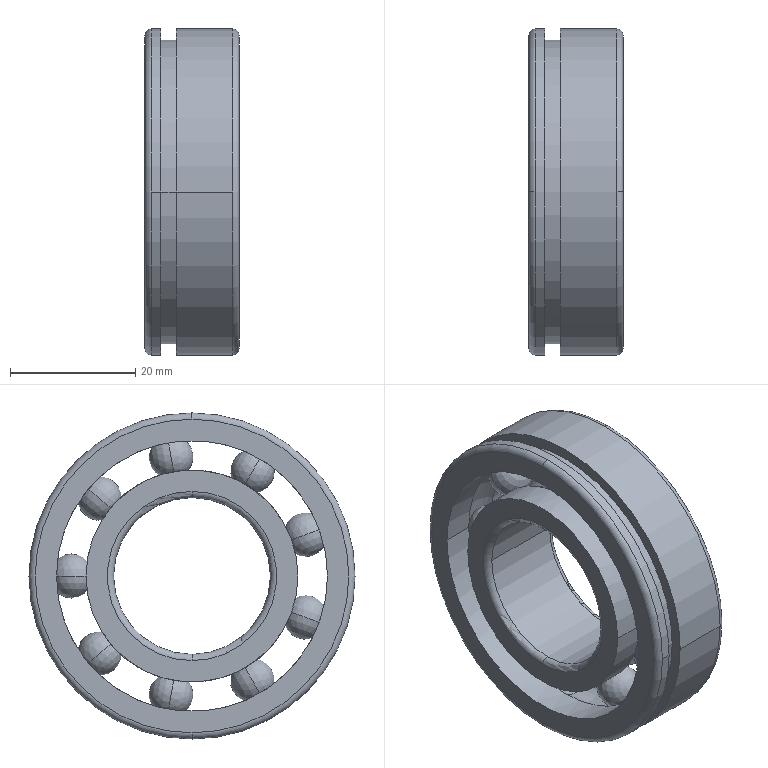Part | SolidWorks | features BaseBody 11 | 11 solids | 54 faces | box 15 x 52 x 52 mm | volume 15772 mm3 | sphere 18 | cylinder 16 | torus 14 | plane 6 | commonest cylinder face diameters 33.802 x4 43.198 x4 52 x4 25 x2 48.4 x2
STEP:
#1=CARTESIAN_POINT('',(7.5,15.74,0.));
#2=VERTEX_POINT('',#1);
#3=CARTESIAN_POINT('',(7.5,22.76,0.));
#4=VERTEX_POINT('',#3);
#5=CARTESIAN_POINT('',(7.5,19.25,0.));
#6=DIRECTION('',(0.,0.,1.));
#7=DIRECTION('',(1.,0.,0.));
#8=AXIS2_PLACEMENT_3D('',#5,#6,#7);
#9=CIRCLE('',#8,3.51);
#10=EDGE_CURVE('',#2,#4,#9,.T.);
#11=ORIENTED_EDGE('',*,*,#10,.F.);
#12=CARTESIAN_POINT('',(7.5,19.25,0.));
#13=DIRECTION('',(0.,0.,-1.));
#14=DIRECTION('',(-1.,0.,0.));
#15=AXIS2_PLACEMENT_3D('',#12,#13,#14);
#16=CIRCLE('',#15,3.51);
#17=EDGE_CURVE('',#2,#4,#16,.T.);
#18=ORIENTED_EDGE('',*,*,#17,.T.);
#19=EDGE_LOOP('',(#11,#18));
#20=FACE_OUTER_BOUND('',#19,.T.);
#21=CARTESIAN_POINT('',(7.5,19.25,0.));
#22=DIRECTION('',(0.,0.,-1.));
#23=DIRECTION('',(1.,0.,0.));
#24=AXIS2_PLACEMENT_3D('',#21,#22,#23);
#25=SPHERICAL_SURFACE('',#24,3.51);
#26=ADVANCED_FACE('',(#20),#25,.T.);
#27=ORIENTED_EDGE('',*,*,#17,.F.);
#28=ORIENTED_EDGE('',*,*,#10,.T.);
#29=EDGE_LOOP('',(#27,#28));
#30=FACE_OUTER_BOUND('',#29,.T.);
#31=CARTESIAN_POINT('',(7.5,19.25,0.));
#32=DIRECTION('',(0.,0.,-1.));
#33=DIRECTION('',(1.,0.,0.));
#34=AXIS2_PLACEMENT_3D('',#31,#32,#33);
#35=SPHERICAL_SURFACE('',#34,3.51);
#36=ADVANCED_FACE('',(#30),#35,.T.);
#37=CLOSED_SHELL('',(#26,#36));
#38=MANIFOLD_SOLID_BREP('',#37);
#39=CARTESIAN_POINT('',(5.,-24.2,0.));
#40=VERTEX_POINT('',#39);
#41=CARTESIAN_POINT('',(5.,24.2,0.));
#42=VERTEX_POINT('',#41);
#43=CARTESIAN_POINT('',(5.,0.,0.));
#44=DIRECTION('',(1.,0.,0.));
#45=DIRECTION('',(0.,1.,0.));
#46=AXIS2_PLACEMENT_3D('',#43,#44,#45);
#47=CIRCLE('',#46,24.2);
#48=EDGE_CURVE('',#40,#42,#47,.T.);
#49=ORIENTED_EDGE('',*,*,#48,.F.);
#50=CARTESIAN_POINT('',(2.5,-24.2,0.));
#51=VERTEX_POINT('',#50);
#52=CARTESIAN_POINT('',(3.75,-24.2,0.));
#53=DIRECTION('',(-1.,0.,0.));
#54=VECTOR('',#53,1000.);
#55=LINE('',#52,#54);
#56=EDGE_CURVE('',#40,#51,#55,.T.);
#57=ORIENTED_EDGE('',*,*,#56,.T.);
#58=CARTESIAN_POINT('',(2.5,24.2,0.));
#59=VERTEX_POINT('',#58);
#60=CARTESIAN_POINT('',(2.5,0.,0.));
#61=DIRECTION('',(1.,0.,0.));
#62=DIRECTION('',(0.,1.,0.));
#63=AXIS2_PLACEMENT_3D('',#60,#61,#62);
#64=CIRCLE('',#63,24.2);
#65=EDGE_CURVE('',#51,#59,#64,.T.);
#66=ORIENTED_EDGE('',*,*,#65,.T.);
#67=CARTESIAN_POINT('',(3.75,24.2,0.));
#68=DIRECTION('',(-1.,0.,0.));
#69=VECTOR('',#68,1000.);
#70=LINE('',#67,#69);
#71=EDGE_CURVE('',#42,#59,#70,.T.);
#72=ORIENTED_EDGE('',*,*,#71,.F.);
#73=EDGE_LOOP('',(#49,#57,#66,#72));
#74=FACE_OUTER_BOUND('',#73,.T.);
#75=CARTESIAN_POINT('',(3.75,0.,0.));
#76=DIRECTION('',(-1.,0.,0.));
#77=DIRECTION('',(0.,1.,0.));
#78=AXIS2_PLACEMENT_3D('',#75,#76,#77);
#79=CYLINDRICAL_SURFACE('',#78,24.2);
#80=ADVANCED_FACE('',(#74),#79,.T.);
#81=CARTESIAN_POINT('',(14.,-26.,0.));
#82=VERTEX_POINT('',#81);
#83=CARTESIAN_POINT('',(14.,0.,-26.));
#84=VERTEX_POINT('',#83);
#85=CARTESIAN_POINT('',(14.,0.,0.));
#86=DIRECTION('',(1.,0.,0.));
#87=DIRECTION('',(0.,-1.,0.));
#88=AXIS2_PLACEMENT_3D('',#85,#86,#87);
#89=CIRCLE('',#88,26.);
#90=EDGE_CURVE('',#82,#84,#89,.T.);
#91=ORIENTED_EDGE('',*,*,#90,.F.);
#92=CARTESIAN_POINT('',(5.,-26.,0.));
#93=VERTEX_POINT('',#92);
#94=CARTESIAN_POINT('',(10.,-26.,0.));
#95=DIRECTION('',(-1.,0.,0.));
#96=VECTOR('',#95,1000.);
#97=LINE('',#94,#96);
#98=EDGE_CURVE('',#82,#93,#97,.T.);
#99=ORIENTED_EDGE('',*,*,#98,.T.);
#100=CARTESIAN_POINT('',(5.,26.,0.));
#101=VERTEX_POINT('',#100);
#102=CARTESIAN_POINT('',(5.,0.,0.));
#103=DIRECTION('',(1.,0.,0.));
#104=DIRECTION('',(0.,1.,0.));
#105=AXIS2_PLACEMENT_3D('',#102,#103,#104);
#106=CIRCLE('',#105,26.);
#107=EDGE_CURVE('',#93,#101,#106,.T.);
#108=ORIENTED_EDGE('',*,*,#107,.T.);
#109=CARTESIAN_POINT('',(14.,26.,0.));
#110=VERTEX_POINT('',#109);
#111=CARTESIAN_POINT('',(10.,26.,0.));
#112=DIRECTION('',(-1.,0.,0.));
#113=VECTOR('',#112,1000.);
#114=LINE('',#111,#113);
#115=EDGE_CURVE('',#110,#101,#114,.T.);
#116=ORIENTED_EDGE('',*,*,#115,.F.);
#117=CARTESIAN_POINT('',(14.,0.,0.));
#118=DIRECTION('',(1.,0.,0.));
#119=DIRECTION('',(0.,-1.,0.));
#120=AXIS2_PLACEMENT_3D('',#117,#118,#119);
#121=CIRCLE('',#120,26.);
#122=EDGE_CURVE('',#84,#110,#121,.T.);
#123=ORIENTED_EDGE('',*,*,#122,.F.);
#124=EDGE_LOOP('',(#91,#99,#108,#116,#123));
#125=FACE_OUTER_BOUND('',#124,.T.);
#126=CARTESIAN_POINT('',(10.,0.,0.));
#127=DIRECTION('',(-1.,0.,0.));
#128=DIRECTION('',(0.,1.,0.));
#129=AXIS2_PLACEMENT_3D('',#126,#127,#128);
#130=CYLINDRICAL_SURFACE('',#129,26.);
#131=ADVANCED_FACE('',(#125),#130,.T.);
#132=CARTESIAN_POINT('',(2.5,-26.,0.));
#133=VERTEX_POINT('',#132);
#134=CARTESIAN_POINT('',(2.5,26.,0.));
#135=VERTEX_POINT('',#134);
#136=CARTESIAN_POINT('',(2.5,0.,0.));
#137=DIRECTION('',(1.,0.,0.));
#138=DIRECTION('',(0.,1.,0.));
#139=AXIS2_PLACEMENT_3D('',#136,#137,#138);
#140=CIRCLE('',#139,26.);
#141=EDGE_CURVE('',#133,#135,#140,.T.);
#142=ORIENTED_EDGE('',*,*,#141,.F.);
#143=CARTESIAN_POINT('',(1.,-26.,0.));
#144=VERTEX_POINT('',#143);
#145=CARTESIAN_POINT('',(1.25,-26.,0.));
#146=DIRECTION('',(-1.,0.,0.));
#147=VECTOR('',#146,1000.);
#148=LINE('',#145,#147);
#149=EDGE_CURVE('',#133,#144,#148,.T.);
#150=ORIENTED_EDGE('',*,*,#149,.T.);
#151=CARTESIAN_POINT('',(1.,0.,-26.));
#152=VERTEX_POINT('',#151);
#153=CARTESIAN_POINT('',(1.,0.,0.));
#154=DIRECTION('',(-1.,0.,0.));
#155=DIRECTION('',(0.,-1.,0.));
#156=AXIS2_PLACEMENT_3D('',#153,#154,#155);
#157=CIRCLE('',#156,26.);
#158=EDGE_CURVE('',#152,#144,#157,.T.);
#159=ORIENTED_EDGE('',*,*,#158,.F.);
#160=CARTESIAN_POINT('',(1.,26.,0.));
#161=VERTEX_POINT('',#160);
#162=CARTESIAN_POINT('',(1.,0.,0.));
#163=DIRECTION('',(-1.,0.,0.));
#164=DIRECTION('',(0.,-1.,0.));
#165=AXIS2_PLACEMENT_3D('',#162,#163,#164);
#166=CIRCLE('',#165,26.);
#167=EDGE_CURVE('',#161,#152,#166,.T.);
#168=ORIENTED_EDGE('',*,*,#167,.F.);
#169=CARTESIAN_POINT('',(1.25,26.,0.));
#170=DIRECTION('',(-1.,0.,0.));
#171=VECTOR('',#170,1000.);
#172=LINE('',#169,#171);
#173=EDGE_CURVE('',#135,#161,#172,.T.);
#174=ORIENTED_EDGE('',*,*,#173,.F.);
#175=EDGE_LOOP('',(#142,#150,#159,#168,#174));
#176=FACE_OUTER_BOUND('',#175,.T.);
#177=CARTESIAN_POINT('',(1.25,0.,0.));
#178=DIRECTION('',(-1.,0.,0.));
#179=DIRECTION('',(0.,1.,0.));
#180=AXIS2_PLACEMENT_3D('',#177,#178,#179);
#181=CYLINDRICAL_SURFACE('',#180,26.);
#182=ADVANCED_FACE('',(#176),#181,.T.);
#183=ORIENTED_EDGE('',*,*,#122,.T.);
#184=CARTESIAN_POINT('',(14.,0.,26.));
#185=VERTEX_POINT('',#184);
#186=CARTESIAN_POINT('',(14.,0.,0.));
#187=DIRECTION('',(1.,0.,0.));
#188=DIRECTION('',(0.,-1.,0.));
#189=AXIS2_PLACEMENT_3D('',#186,#187,#188);
#190=CIRCLE('',#189,26.);
#191=EDGE_CURVE('',#110,#185,#190,.T.);
#192=ORIENTED_EDGE('',*,*,#191,.T.);
#193=CARTESIAN_POINT('',(15.,0.,25.));
#194=VERTEX_POINT('',#193);
#195=CARTESIAN_POINT('',(14.,0.,25.));
#196=DIRECTION('',(0.,1.,0.));
#197=DIRECTION('',(0.,0.,1.));
#198=AXIS2_PLACEMENT_3D('',#195,#196,#197);
#199=CIRCLE('',#198,1.);
#200=EDGE_CURVE('',#185,#194,#199,.T.);
#201=ORIENTED_EDGE('',*,*,#200,.T.);
#202=CARTESIAN_POINT('',(15.,0.,-25.));
#203=VERTEX_POINT('',#202);
#204=CARTESIAN_POINT('',(15.,0.,0.));
#205=DIRECTION('',(-1.,0.,0.));
#206=DIRECTION('',(0.,-1.,0.));
#207=AXIS2_PLACEMENT_3D('',#204,#205,#206);
#208=CIRCLE('',#207,25.);
#209=EDGE_CURVE('',#194,#203,#208,.T.);
#210=ORIENTED_EDGE('',*,*,#209,.T.);
#211=CARTESIAN_POINT('',(14.,0.,-25.));
#212=DIRECTION('',(0.,-1.,0.));
#213=DIRECTION('',(0.,0.,-1.));
#214=AXIS2_PLACEMENT_3D('',#211,#212,#213);
#215=CIRCLE('',#214,1.);
#216=EDGE_CURVE('',#84,#203,#215,.T.);
#217=ORIENTED_EDGE('',*,*,#216,.F.);
#218=EDGE_LOOP('',(#183,#192,#201,#210,#217));
#219=FACE_OUTER_BOUND('',#218,.T.);
#220=CARTESIAN_POINT('',(14.,0.,0.));
#221=DIRECTION('',(1.,0.,0.));
#222=DIRECTION('',(0.,0.,-1.));
#223=AXIS2_PLACEMENT_3D('',#220,#221,#222);
#224=TOROIDAL_SURFACE('',#223,25.,1.);
#225=ADVANCED_FACE('',(#219),#224,.T.);
#226=CARTESIAN_POINT('',(0.,0.,-25.));
#227=VERTEX_POINT('',#226);
#228=CARTESIAN_POINT('',(0.,0.,25.));
#229=VERTEX_POINT('',#228);
#230=CARTESIAN_POINT('',(0.,0.,0.));
#231=DIRECTION('',(1.,0.,0.));
#232=DIRECTION('',(0.,-1.,0.));
#233=AXIS2_PLACEMENT_3D('',#230,#231,#232);
#234=CIRCLE('',#233,25.);
#235=EDGE_CURVE('',#227,#229,#234,.T.);
#236=ORIENTED_EDGE('',*,*,#235,.T.);
#237=CARTESIAN_POINT('',(1.,0.,26.));
#238=VERTEX_POINT('',#237);
#239=CARTESIAN_POINT('',(1.,0.,25.));
#240=DIRECTION('',(0.,1.,0.));
#241=DIRECTION('',(0.,0.,1.));
#242=AXIS2_PLACEMENT_3D('',#239,#240,#241);
#243=CIRCLE('',#242,1.);
#244=EDGE_CURVE('',#229,#238,#243,.T.);
#245=ORIENTED_EDGE('',*,*,#244,.T.);
#246=CARTESIAN_POINT('',(1.,0.,0.));
#247=DIRECTION('',(-1.,0.,0.));
#248=DIRECTION('',(0.,-1.,0.));
#249=AXIS2_PLACEMENT_3D('',#246,#247,#248);
#250=CIRCLE('',#249,26.);
#251=EDGE_CURVE('',#238,#161,#250,.T.);
#252=ORIENTED_EDGE('',*,*,#251,.T.);
#253=ORIENTED_EDGE('',*,*,#167,.T.);
#254=CARTESIAN_POINT('',(1.,0.,-25.));
#255=DIRECTION('',(0.,-1.,0.));
#256=DIRECTION('',(0.,0.,-1.));
#257=AXIS2_PLACEMENT_3D('',#254,#255,#256);
#258=CIRCLE('',#257,1.);
#259=EDGE_CURVE('',#227,#152,#258,.T.);
#260=ORIENTED_EDGE('',*,*,#259,.F.);
#261=EDGE_LOOP('',(#236,#245,#252,#253,#260));
#262=FACE_OUTER_BOUND('',#261,.T.);
#263=CARTESIAN_POINT('',(1.,0.,0.));
#264=DIRECTION('',(1.,0.,0.));
#265=DIRECTION('',(0.,0.,-1.));
#266=AXIS2_PLACEMENT_3D('',#263,#264,#265);
#267=TOROIDAL_SURFACE('',#266,25.,1.);
#268=ADVANCED_FACE('',(#262),#267,.T.);
#269=CARTESIAN_POINT('',(4.892,0.,21.599));
#270=VERTEX_POINT('',#269);
#271=CARTESIAN_POINT('',(4.892,-21.599,0.));
#272=VERTEX_POINT('',#271);
#273=CARTESIAN_POINT('',(4.892,0.,0.));
#274=DIRECTION('',(1.,0.,0.));
#275=DIRECTION('',(0.,1.,0.));
#276=AXIS2_PLACEMENT_3D('',#273,#274,#275);
#277=CIRCLE('',#276,21.599);
#278=EDGE_CURVE('',#270,#272,#277,.T.);
#279=ORIENTED_EDGE('',*,*,#278,.F.);
#280=CARTESIAN_POINT('',(10.108,0.,21.599));
#281=VERTEX_POINT('',#280);
#282=CARTESIAN_POINT('',(7.5,0.,19.25));
#283=DIRECTION('',(0.,1.,0.));
#284=DIRECTION('',(0.,0.,1.));
#285=AXIS2_PLACEMENT_3D('',#282,#283,#284);
#286=CIRCLE('',#285,3.51);
#287=EDGE_CURVE('',#270,#281,#286,.T.);
#288=ORIENTED_EDGE('',*,*,#287,.T.);
#289=CARTESIAN_POINT('',(10.108,-21.599,0.));
#290=VERTEX_POINT('',#289);
#291=CARTESIAN_POINT('',(10.108,0.,0.));
#292=DIRECTION('',(1.,0.,0.));
#293=DIRECTION('',(0.,1.,0.));
#294=AXIS2_PLACEMENT_3D('',#291,#292,#293);
#295=CIRCLE('',#294,21.599);
#296=EDGE_CURVE('',#281,#290,#295,.T.);
#297=ORIENTED_EDGE('',*,*,#296,.T.);
#298=CARTESIAN_POINT('',(10.108,0.,-21.599));
#299=VERTEX_POINT('',#298);
#300=CARTESIAN_POINT('',(10.108,0.,0.));
#301=DIRECTION('',(1.,0.,0.));
#302=DIRECTION('',(0.,1.,0.));
#303=AXIS2_PLACEMENT_3D('',#300,#301,#302);
#304=CIRCLE('',#303,21.599);
#305=EDGE_CURVE('',#290,#299,#304,.T.);
#306=ORIENTED_EDGE('',*,*,#305,.T.);
#307=CARTESIAN_POINT('',(4.892,0.,-21.599));
#308=VERTEX_POINT('',#307);
#309=CARTESIAN_POINT('',(7.5,0.,-19.25));
#310=DIRECTION('',(0.,-1.,0.));
#311=DIRECTION('',(0.,0.,-1.));
#312=AXIS2_PLACEMENT_3D('',#309,#310,#311);
#313=CIRCLE('',#312,3.51);
#314=EDGE_CURVE('',#308,#299,#313,.T.);
#315=ORIENTED_EDGE('',*,*,#314,.F.);
#316=CARTESIAN_POINT('',(4.892,0.,0.));
#317=DIRECTION('',(1.,0.,0.));
#318=DIRECTION('',(0.,1.,0.));
#319=AXIS2_PLACEMENT_3D('',#316,#317,#318);
#320=CIRCLE('',#319,21.599);
#321=EDGE_CURVE('',#272,#308,#320,.T.);
#322=ORIENTED_EDGE('',*,*,#321,.F.);
#323=EDGE_LOOP('',(#279,#288,#297,#306,#315,#322));
#324=FACE_OUTER_BOUND('',#323,.T.);
#325=CARTESIAN_POINT('',(7.5,0.,0.));
#326=DIRECTION('',(1.,0.,0.));
#327=DIRECTION('',(0.,0.,-1.));
#328=AXIS2_PLACEMENT_3D('',#325,#326,#327);
#329=TOROIDAL_SURFACE('',#328,19.25,3.51);
#330=ADVANCED_FACE('',(#324),#329,.F.);
#331=CARTESIAN_POINT('',(15.,21.599,0.));
#332=VERTEX_POINT('',#331);
#333=CARTESIAN_POINT('',(15.,-21.599,0.));
#334=VERTEX_POINT('',#333);
#335=CARTESIAN_POINT('',(15.,0.,0.));
#336=DIRECTION('',(1.,0.,0.));
#337=DIRECTION('',(0.,1.,0.));
#338=AXIS2_PLACEMENT_3D('',#335,#336,#337);
#339=CIRCLE('',#338,21.599);
#340=EDGE_CURVE('',#332,#334,#339,.T.);
#341=ORIENTED_EDGE('',*,*,#340,.T.);
#342=CARTESIAN_POINT('',(12.554,-21.599,0.));
#343=DIRECTION('',(-1.,0.,0.));
#344=VECTOR('',#343,1000.);
#345=LINE('',#342,#344);
#346=EDGE_CURVE('',#334,#290,#345,.T.);
#347=ORIENTED_EDGE('',*,*,#346,.T.);
#348=ORIENTED_EDGE('',*,*,#296,.F.);
#349=CARTESIAN_POINT('',(10.108,21.599,0.));
#350=VERTEX_POINT('',#349);
#351=CARTESIAN_POINT('',(10.108,0.,0.));
#352=DIRECTION('',(1.,0.,0.));
#353=DIRECTION('',(0.,1.,0.));
#354=AXIS2_PLACEMENT_3D('',#351,#352,#353);
#355=CIRCLE('',#354,21.599);
#356=EDGE_CURVE('',#350,#281,#355,.T.);
#357=ORIENTED_EDGE('',*,*,#356,.F.);
#358=CARTESIAN_POINT('',(12.554,21.599,0.));
#359=DIRECTION('',(-1.,0.,0.));
#360=VECTOR('',#359,1000.);
#361=LINE('',#358,#360);
#362=EDGE_CURVE('',#332,#350,#361,.T.);
#363=ORIENTED_EDGE('',*,*,#362,.F.);
#364=EDGE_LOOP('',(#341,#347,#348,#357,#363));
#365=FACE_OUTER_BOUND('',#364,.T.);
#366=CARTESIAN_POINT('',(12.554,0.,0.));
#367=DIRECTION('',(-1.,0.,0.));
#368=DIRECTION('',(0.,1.,0.));
#369=AXIS2_PLACEMENT_3D('',#366,#367,#368);
#370=CYLINDRICAL_SURFACE('',#369,21.599);
#371=ADVANCED_FACE('',(#365),#370,.F.);
#372=CARTESIAN_POINT('',(4.892,21.599,0.));
#373=VERTEX_POINT('',#372);
#374=CARTESIAN_POINT('',(4.892,0.,0.));
#375=DIRECTION('',(1.,0.,0.));
#376=DIRECTION('',(0.,1.,0.));
#377=AXIS2_PLACEMENT_3D('',#374,#375,#376);
#378=CIRCLE('',#377,21.599);
#379=EDGE_CURVE('',#373,#270,#378,.T.);
#380=ORIENTED_EDGE('',*,*,#379,.T.);
#381=ORIENTED_EDGE('',*,*,#278,.T.);
#382=CARTESIAN_POINT('',(0.,-21.599,0.));
#383=VERTEX_POINT('',#382);
#384=CARTESIAN_POINT('',(2.446,-21.599,0.));
#385=DIRECTION('',(-1.,0.,0.));
#386=VECTOR('',#385,1000.);
#387=LINE('',#384,#386);
#388=EDGE_CURVE('',#272,#383,#387,.T.);
#389=ORIENTED_EDGE('',*,*,#388,.T.);
#390=CARTESIAN_POINT('',(0.,21.599,0.));
#391=VERTEX_POINT('',#390);
#392=CARTESIAN_POINT('',(0.,0.,0.));
#393=DIRECTION('',(1.,0.,0.));
#394=DIRECTION('',(0.,1.,0.));
#395=AXIS2_PLACEMENT_3D('',#392,#393,#394);
#396=CIRCLE('',#395,21.599);
#397=EDGE_CURVE('',#391,#383,#396,.T.);
#398=ORIENTED_EDGE('',*,*,#397,.F.);
#399=CARTESIAN_POINT('',(2.446,21.599,0.));
#400=DIRECTION('',(-1.,0.,0.));
#401=VECTOR('',#400,1000.);
#402=LINE('',#399,#401);
#403=EDGE_CURVE('',#373,#391,#402,.T.);
#404=ORIENTED_EDGE('',*,*,#403,.F.);
#405=EDGE_LOOP('',(#380,#381,#389,#398,#404));
#406=FACE_OUTER_BOUND('',#405,.T.);
#407=CARTESIAN_POINT('',(2.446,0.,0.));
#408=DIRECTION('',(-1.,0.,0.));
#409=DIRECTION('',(0.,1.,0.));
#410=AXIS2_PLACEMENT_3D('',#407,#408,#409);
#411=CYLINDRICAL_SURFACE('',#410,21.599);
#412=ADVANCED_FACE('',(#406),#411,.F.);
#413=CARTESIAN_POINT('',(5.,0.,0.));
#414=DIRECTION('',(1.,0.,0.));
#415=DIRECTION('',(0.,1.,0.));
#416=AXIS2_PLACEMENT_3D('',#413,#414,#415);
#417=CIRCLE('',#416,24.2);
#418=EDGE_CURVE('',#42,#40,#417,.T.);
#419=ORIENTED_EDGE('',*,*,#418,.T.);
#420=ORIENTED_EDGE('',*,*,#48,.T.);
#421=EDGE_LOOP('',(#419,#420));
#422=FACE_BOUND('',#421,.T.);
#423=CARTESIAN_POINT('',(5.,0.,0.));
#424=DIRECTION('',(1.,0.,0.));
#425=DIRECTION('',(0.,1.,0.));
#426=AXIS2_PLACEMENT_3D('',#423,#424,#425);
#427=CIRCLE('',#426,26.);
#428=EDGE_CURVE('',#101,#93,#427,.T.);
#429=ORIENTED_EDGE('',*,*,#428,.F.);
#430=ORIENTED_EDGE('',*,*,#107,.F.);
#431=EDGE_LOOP('',(#429,#430));
#432=FACE_OUTER_BOUND('',#431,.T.);
#433=CARTESIAN_POINT('',(5.,25.1,0.));
#434=DIRECTION('',(-1.,0.,0.));
#435=DIRECTION('',(0.,0.,1.));
#436=AXIS2_PLACEMENT_3D('',#433,#434,#435);
#437=PLANE('',#436);
#438=ADVANCED_FACE('',(#422,#432),#437,.T.);
#439=CARTESIAN_POINT('',(2.5,0.,0.));
#440=DIRECTION('',(1.,0.,0.));
#441=DIRECTION('',(0.,1.,0.));
#442=AXIS2_PLACEMENT_3D('',#439,#440,#441);
#443=CIRCLE('',#442,24.2);
#444=EDGE_CURVE('',#59,#51,#443,.T.);
#445=ORIENTED_EDGE('',*,*,#444,.F.);
#446=ORIENTED_EDGE('',*,*,#65,.F.);
#447=EDGE_LOOP('',(#445,#446));
#448=FACE_BOUND('',#447,.T.);
#449=CARTESIAN_POINT('',(2.5,0.,0.));
#450=DIRECTION('',(1.,0.,0.));
#451=DIRECTION('',(0.,1.,0.));
#452=AXIS2_PLACEMENT_3D('',#449,#450,#451);
#453=CIRCLE('',#452,26.);
#454=EDGE_CURVE('',#135,#133,#453,.T.);
#455=ORIENTED_EDGE('',*,*,#454,.T.);
#456=ORIENTED_EDGE('',*,*,#141,.T.);
#457=EDGE_LOOP('',(#455,#456));
#458=FACE_OUTER_BOUND('',#457,.T.);
#459=CARTESIAN_POINT('',(2.5,25.1,0.));
#460=DIRECTION('',(1.,0.,0.));
#461=DIRECTION('',(0.,1.,0.));
#462=AXIS2_PLACEMENT_3D('',#459,#460,#461);
#463=PLANE('',#462);
#464=ADVANCED_FACE('',(#448,#458),#463,.T.);
#465=ORIENTED_EDGE('',*,*,#340,.F.);
#466=CARTESIAN_POINT('',(15.,0.,0.));
#467=DIRECTION('',(1.,0.,0.));
#468=DIRECTION('',(0.,1.,0.));
#469=AXIS2_PLACEMENT_3D('',#466,#467,#468);
#470=CIRCLE('',#469,21.599);
#471=EDGE_CURVE('',#334,#332,#470,.T.);
#472=ORIENTED_EDGE('',*,*,#471,.F.);
#473=EDGE_LOOP('',(#465,#472));
#474=FACE_BOUND('',#473,.T.);
#475=CARTESIAN_POINT('',(15.,0.,0.));
#476=DIRECTION('',(-1.,0.,0.));
#477=DIRECTION('',(0.,-1.,0.));
#478=AXIS2_PLACEMENT_3D('',#475,#476,#477);
#479=CIRCLE('',#478,25.);
#480=EDGE_CURVE('',#203,#194,#479,.T.);
#481=ORIENTED_EDGE('',*,*,#480,.F.);
#482=ORIENTED_EDGE('',*,*,#209,.F.);
#483=EDGE_LOOP('',(#481,#482));
#484=FACE_OUTER_BOUND('',#483,.T.);
#485=CARTESIAN_POINT('',(15.,23.8,0.));
#486=DIRECTION('',(1.,0.,0.));
#487=DIRECTION('',(0.,1.,0.));
#488=AXIS2_PLACEMENT_3D('',#485,#486,#487);
#489=PLANE('',#488);
#490=ADVANCED_FACE('',(#474,#484),#489,.T.);
#491=ORIENTED_EDGE('',*,*,#397,.T.);
#492=CARTESIAN_POINT('',(0.,0.,0.));
#493=DIRECTION('',(1.,0.,0.));
#494=DIRECTION('',(0.,1.,0.));
#495=AXIS2_PLACEMENT_3D('',#492,#493,#494);
#496=CIRCLE('',#495,21.599);
#497=EDGE_CURVE('',#383,#391,#496,.T.);
#498=ORIENTED_EDGE('',*,*,#497,.T.);
#499=EDGE_LOOP('',(#491,#498));
#500=FACE_BOUND('',#499,.T.);
#501=ORIENTED_EDGE('',*,*,#235,.F.);
#502=CARTESIAN_POINT('',(0.,0.,0.));
#503=DIRECTION('',(1.,0.,0.));
#504=DIRECTION('',(0.,-1.,0.));
#505=AXIS2_PLACEMENT_3D('',#502,#503,#504);
#506=CIRCLE('',#505,25.);
#507=EDGE_CURVE('',#229,#227,#506,.T.);
#508=ORIENTED_EDGE('',*,*,#507,.F.);
#509=EDGE_LOOP('',(#501,#508));
#510=FACE_OUTER_BOUND('',#509,.T.);
#511=CARTESIAN_POINT('',(0.,23.8,0.));
#512=DIRECTION('',(-1.,0.,0.));
#513=DIRECTION('',(0.,0.,1.));
#514=AXIS2_PLACEMENT_3D('',#511,#512,#513);
#515=PLANE('',#514);
#516=ADVANCED_FACE('',(#500,#510),#515,.T.);
#517=ORIENTED_EDGE('',*,*,#388,.F.);
#518=ORIENTED_EDGE('',*,*,#321,.T.);
#519=CARTESIAN_POINT('',(4.892,0.,0.));
#520=DIRECTION('',(1.,0.,0.));
#521=DIRECTION('',(0.,1.,0.));
#522=AXIS2_PLACEMENT_3D('',#519,#520,#521);
#523=CIRCLE('',#522,21.599);
#524=EDGE_CURVE('',#308,#373,#523,.T.);
#525=ORIENTED_EDGE('',*,*,#524,.T.);
#526=ORIENTED_EDGE('',*,*,#403,.T.);
#527=ORIENTED_EDGE('',*,*,#497,.F.);
#528=EDGE_LOOP('',(#517,#518,#525,#526,#527));
#529=FACE_OUTER_BOUND('',#528,.T.);
#530=CARTESIAN_POINT('',(2.446,0.,0.));
#531=DIRECTION('',(-1.,0.,0.));
#532=DIRECTION('',(0.,1.,0.));
#533=AXIS2_PLACEMENT_3D('',#530,#531,#532);
#534=CYLINDRICAL_SURFACE('',#533,21.599);
#535=ADVANCED_FACE('',(#529),#534,.F.);
#536=ORIENTED_EDGE('',*,*,#346,.F.);
#537=ORIENTED_EDGE('',*,*,#471,.T.);
#538=ORIENTED_EDGE('',*,*,#362,.T.);
#539=CARTESIAN_POINT('',(10.108,0.,0.));
#540=DIRECTION('',(1.,0.,0.));
#541=DIRECTION('',(0.,1.,0.));
#542=AXIS2_PLACEMENT_3D('',#539,#540,#541);
#543=CIRCLE('',#542,21.599);
#544=EDGE_CURVE('',#299,#350,#543,.T.);
#545=ORIENTED_EDGE('',*,*,#544,.F.);
#546=ORIENTED_EDGE('',*,*,#305,.F.);
#547=EDGE_LOOP('',(#536,#537,#538,#545,#546));
#548=FACE_OUTER_BOUND('',#547,.T.);
#549=CARTESIAN_POINT('',(12.554,0.,0.));
#550=DIRECTION('',(-1.,0.,0.));
#551=DIRECTION('',(0.,1.,0.));
#552=AXIS2_PLACEMENT_3D('',#549,#550,#551);
#553=CYLINDRICAL_SURFACE('',#552,21.599);
#554=ADVANCED_FACE('',(#548),#553,.F.);
#555=ORIENTED_EDGE('',*,*,#287,.F.);
#556=ORIENTED_EDGE('',*,*,#379,.F.);
#557=ORIENTED_EDGE('',*,*,#524,.F.);
#558=ORIENTED_EDGE('',*,*,#314,.T.);
#559=ORIENTED_EDGE('',*,*,#544,.T.);
#560=ORIENTED_EDGE('',*,*,#356,.T.);
#561=EDGE_LOOP('',(#555,#556,#557,#558,#559,#560));
#562=FACE_OUTER_BOUND('',#561,.T.);
#563=CARTESIAN_POINT('',(7.5,0.,0.));
#564=DIRECTION('',(1.,0.,0.));
#565=DIRECTION('',(0.,0.,-1.));
#566=AXIS2_PLACEMENT_3D('',#563,#564,#565);
#567=TOROIDAL_SURFACE('',#566,19.25,3.51);
#568=ADVANCED_FACE('',(#562),#567,.F.);
#569=ORIENTED_EDGE('',*,*,#244,.F.);
#570=ORIENTED_EDGE('',*,*,#507,.T.);
#571=ORIENTED_EDGE('',*,*,#259,.T.);
#572=ORIENTED_EDGE('',*,*,#158,.T.);
#573=CARTESIAN_POINT('',(1.,0.,0.));
#574=DIRECTION('',(-1.,0.,0.));
#575=DIRECTION('',(0.,-1.,0.));
#576=AXIS2_PLACEMENT_3D('',#573,#574,#575);
#577=CIRCLE('',#576,26.);
#578=EDGE_CURVE('',#144,#238,#577,.T.);
#579=ORIENTED_EDGE('',*,*,#578,.T.);
#580=EDGE_LOOP('',(#569,#570,#571,#572,#579));
#581=FACE_OUTER_BOUND('',#580,.T.);
#582=CARTESIAN_POINT('',(1.,0.,0.));
#583=DIRECTION('',(1.,0.,0.));
#584=DIRECTION('',(0.,0.,-1.));
#585=AXIS2_PLACEMENT_3D('',#582,#583,#584);
#586=TOROIDAL_SURFACE('',#585,25.,1.);
#587=ADVANCED_FACE('',(#581),#586,.T.);
#588=ORIENTED_EDGE('',*,*,#200,.F.);
#589=CARTESIAN_POINT('',(14.,0.,0.));
#590=DIRECTION('',(1.,0.,0.));
#591=DIRECTION('',(0.,-1.,0.));
#592=AXIS2_PLACEMENT_3D('',#589,#590,#591);
#593=CIRCLE('',#592,26.);
#594=EDGE_CURVE('',#185,#82,#593,.T.);
#595=ORIENTED_EDGE('',*,*,#594,.T.);
#596=ORIENTED_EDGE('',*,*,#90,.T.);
#597=ORIENTED_EDGE('',*,*,#216,.T.);
#598=ORIENTED_EDGE('',*,*,#480,.T.);
#599=EDGE_LOOP('',(#588,#595,#596,#597,#598));
#600=FACE_OUTER_BOUND('',#599,.T.);
#601=CARTESIAN_POINT('',(14.,0.,0.));
#602=DIRECTION('',(1.,0.,0.));
#603=DIRECTION('',(0.,0.,-1.));
#604=AXIS2_PLACEMENT_3D('',#601,#602,#603);
#605=TOROIDAL_SURFACE('',#604,25.,1.);
#606=ADVANCED_FACE('',(#600),#605,.T.);
#607=ORIENTED_EDGE('',*,*,#149,.F.);
#608=ORIENTED_EDGE('',*,*,#454,.F.);
#609=ORIENTED_EDGE('',*,*,#173,.T.);
#610=ORIENTED_EDGE('',*,*,#251,.F.);
#611=ORIENTED_EDGE('',*,*,#578,.F.);
#612=EDGE_LOOP('',(#607,#608,#609,#610,#611));
#613=FACE_OUTER_BOUND('',#612,.T.);
#614=CARTESIAN_POINT('',(1.25,0.,0.));
#615=DIRECTION('',(-1.,0.,0.));
#616=DIRECTION('',(0.,1.,0.));
#617=AXIS2_PLACEMENT_3D('',#614,#615,#616);
#618=CYLINDRICAL_SURFACE('',#617,26.);
#619=ADVANCED_FACE('',(#613),#618,.T.);
#620=ORIENTED_EDGE('',*,*,#98,.F.);
#621=ORIENTED_EDGE('',*,*,#594,.F.);
#622=ORIENTED_EDGE('',*,*,#191,.F.);
#623=ORIENTED_EDGE('',*,*,#115,.T.);
#624=ORIENTED_EDGE('',*,*,#428,.T.);
#625=EDGE_LOOP('',(#620,#621,#622,#623,#624));
#626=FACE_OUTER_BOUND('',#625,.T.);
#627=CARTESIAN_POINT('',(10.,0.,0.));
#628=DIRECTION('',(-1.,0.,0.));
#629=DIRECTION('',(0.,1.,0.));
#630=AXIS2_PLACEMENT_3D('',#627,#628,#629);
#631=CYLINDRICAL_SURFACE('',#630,26.);
#632=ADVANCED_FACE('',(#626),#631,.T.);
#633=ORIENTED_EDGE('',*,*,#56,.F.);
#634=ORIENTED_EDGE('',*,*,#418,.F.);
#635=ORIENTED_EDGE('',*,*,#71,.T.);
#636=ORIENTED_EDGE('',*,*,#444,.T.);
#637=EDGE_LOOP('',(#633,#634,#635,#636));
#638=FACE_OUTER_BOUND('',#637,.T.);
#639=CARTESIAN_POINT('',(3.75,0.,0.));
#640=DIRECTION('',(-1.,0.,0.));
#641=DIRECTION('',(0.,1.,0.));
#642=AXIS2_PLACEMENT_3D('',#639,#640,#641);
#643=CYLINDRICAL_SURFACE('',#642,24.2);
#644=ADVANCED_FACE('',(#638),#643,.T.);
#645=CLOSED_SHELL('',(#80,#131,#182,#225,#268,#330,#371,#412,#438,#464,#490,#516,#535,#554,#568,#587,#606,#619,#632,#644));
#646=MANIFOLD_SOLID_BREP('',#645);
#647=CARTESIAN_POINT('',(10.108,0.,-16.901));
#648=VERTEX_POINT('',#647);
#649=CARTESIAN_POINT('',(7.5,0.,-15.74));
#650=VERTEX_POINT('',#649);
#651=CARTESIAN_POINT('',(7.5,0.,-19.25));
#652=DIRECTION('',(0.,-1.,0.));
#653=DIRECTION('',(0.,0.,-1.));
#654=AXIS2_PLACEMENT_3D('',#651,#652,#653);
#655=CIRCLE('',#654,3.51);
#656=EDGE_CURVE('',#648,#650,#655,.T.);
#657=ORIENTED_EDGE('',*,*,#656,.T.);
#658=CARTESIAN_POINT('',(7.5,0.,15.74));
#659=VERTEX_POINT('',#658);
#660=CARTESIAN_POINT('',(7.5,0.,0.));
#661=DIRECTION('',(1.,0.,0.));
#662=DIRECTION('',(0.,0.,-1.));
#663=AXIS2_PLACEMENT_3D('',#660,#661,#662);
#664=CIRCLE('',#663,15.74);
#665=EDGE_CURVE('',#650,#659,#664,.T.);
#666=ORIENTED_EDGE('',*,*,#665,.T.);
#667=CARTESIAN_POINT('',(10.108,0.,16.901));
#668=VERTEX_POINT('',#667);
#669=CARTESIAN_POINT('',(7.5,0.,19.25));
#670=DIRECTION('',(0.,1.,0.));
#671=DIRECTION('',(0.,0.,1.));
#672=AXIS2_PLACEMENT_3D('',#669,#670,#671);
#673=CIRCLE('',#672,3.51);
#674=EDGE_CURVE('',#668,#659,#673,.T.);
#675=ORIENTED_EDGE('',*,*,#674,.F.);
#676=CARTESIAN_POINT('',(10.108,16.901,0.));
#677=VERTEX_POINT('',#676);
#678=CARTESIAN_POINT('',(10.108,0.,0.));
#679=DIRECTION('',(1.,0.,0.));
#680=DIRECTION('',(0.,1.,0.));
#681=AXIS2_PLACEMENT_3D('',#678,#679,#680);
#682=CIRCLE('',#681,16.901);
#683=EDGE_CURVE('',#677,#668,#682,.T.);
#684=ORIENTED_EDGE('',*,*,#683,.F.);
#685=CARTESIAN_POINT('',(10.108,0.,0.));
#686=DIRECTION('',(1.,0.,0.));
#687=DIRECTION('',(0.,1.,0.));
#688=AXIS2_PLACEMENT_3D('',#685,#686,#687);
#689=CIRCLE('',#688,16.901);
#690=EDGE_CURVE('',#648,#677,#689,.T.);
#691=ORIENTED_EDGE('',*,*,#690,.F.);
#692=EDGE_LOOP('',(#657,#666,#675,#684,#691));
#693=FACE_OUTER_BOUND('',#692,.T.);
#694=CARTESIAN_POINT('',(7.5,0.,0.));
#695=DIRECTION('',(1.,0.,0.));
#696=DIRECTION('',(0.,0.,-1.));
#697=AXIS2_PLACEMENT_3D('',#694,#695,#696);
#698=TOROIDAL_SURFACE('',#697,19.25,3.51);
#699=ADVANCED_FACE('',(#693),#698,.F.);
#700=ORIENTED_EDGE('',*,*,#674,.T.);
#701=CARTESIAN_POINT('',(7.5,0.,0.));
#702=DIRECTION('',(1.,0.,0.));
#703=DIRECTION('',(0.,0.,-1.));
#704=AXIS2_PLACEMENT_3D('',#701,#702,#703);
#705=CIRCLE('',#704,15.74);
#706=EDGE_CURVE('',#659,#650,#705,.T.);
#707=ORIENTED_EDGE('',*,*,#706,.T.);
#708=ORIENTED_EDGE('',*,*,#656,.F.);
#709=CARTESIAN_POINT('',(10.108,-16.901,0.));
#710=VERTEX_POINT('',#709);
#711=CARTESIAN_POINT('',(10.108,0.,0.));
#712=DIRECTION('',(1.,0.,0.));
#713=DIRECTION('',(0.,1.,0.));
#714=AXIS2_PLACEMENT_3D('',#711,#712,#713);
#715=CIRCLE('',#714,16.901);
#716=EDGE_CURVE('',#710,#648,#715,.T.);
#717=ORIENTED_EDGE('',*,*,#716,.F.);
#718=CARTESIAN_POINT('',(10.108,0.,0.));
#719=DIRECTION('',(1.,0.,0.));
#720=DIRECTION('',(0.,1.,0.));
#721=AXIS2_PLACEMENT_3D('',#718,#719,#720);
#722=CIRCLE('',#721,16.901);
#723=EDGE_CURVE('',#668,#710,#722,.T.);
#724=ORIENTED_EDGE('',*,*,#723,.F.);
#725=EDGE_LOOP('',(#700,#707,#708,#717,#724));
#726=FACE_OUTER_BOUND('',#725,.T.);
#727=CARTESIAN_POINT('',(7.5,0.,0.));
#728=DIRECTION('',(1.,0.,0.));
#729=DIRECTION('',(0.,0.,-1.));
#730=AXIS2_PLACEMENT_3D('',#727,#728,#729);
#731=TOROIDAL_SURFACE('',#730,19.25,3.51);
#732=ADVANCED_FACE('',(#726),#731,.F.);
#733=ORIENTED_EDGE('',*,*,#706,.F.);
#734=CARTESIAN_POINT('',(4.892,0.,16.901));
#735=VERTEX_POINT('',#734);
#736=CARTESIAN_POINT('',(7.5,0.,19.25));
#737=DIRECTION('',(0.,1.,0.));
#738=DIRECTION('',(0.,0.,1.));
#739=AXIS2_PLACEMENT_3D('',#736,#737,#738);
#740=CIRCLE('',#739,3.51);
#741=EDGE_CURVE('',#659,#735,#740,.T.);
#742=ORIENTED_EDGE('',*,*,#741,.T.);
#743=CARTESIAN_POINT('',(4.892,-16.901,0.));
#744=VERTEX_POINT('',#743);
#745=CARTESIAN_POINT('',(4.892,0.,0.));
#746=DIRECTION('',(1.,0.,0.));
#747=DIRECTION('',(0.,1.,0.));
#748=AXIS2_PLACEMENT_3D('',#745,#746,#747);
#749=CIRCLE('',#748,16.901);
#750=EDGE_CURVE('',#735,#744,#749,.T.);
#751=ORIENTED_EDGE('',*,*,#750,.T.);
#752=CARTESIAN_POINT('',(4.892,0.,-16.901));
#753=VERTEX_POINT('',#752);
#754=CARTESIAN_POINT('',(4.892,0.,0.));
#755=DIRECTION('',(1.,0.,0.));
#756=DIRECTION('',(0.,1.,0.));
#757=AXIS2_PLACEMENT_3D('',#754,#755,#756);
#758=CIRCLE('',#757,16.901);
#759=EDGE_CURVE('',#744,#753,#758,.T.);
#760=ORIENTED_EDGE('',*,*,#759,.T.);
#761=CARTESIAN_POINT('',(7.5,0.,-19.25));
#762=DIRECTION('',(0.,-1.,0.));
#763=DIRECTION('',(0.,0.,-1.));
#764=AXIS2_PLACEMENT_3D('',#761,#762,#763);
#765=CIRCLE('',#764,3.51);
#766=EDGE_CURVE('',#650,#753,#765,.T.);
#767=ORIENTED_EDGE('',*,*,#766,.F.);
#768=EDGE_LOOP('',(#733,#742,#751,#760,#767));
#769=FACE_OUTER_BOUND('',#768,.T.);
#770=CARTESIAN_POINT('',(7.5,0.,0.));
#771=DIRECTION('',(1.,0.,0.));
#772=DIRECTION('',(0.,0.,-1.));
#773=AXIS2_PLACEMENT_3D('',#770,#771,#772);
#774=TOROIDAL_SURFACE('',#773,19.25,3.51);
#775=ADVANCED_FACE('',(#769),#774,.F.);
#776=CARTESIAN_POINT('',(14.,-12.5,0.));
#777=VERTEX_POINT('',#776);
#778=CARTESIAN_POINT('',(14.,0.,12.5));
#779=VERTEX_POINT('',#778);
#780=CARTESIAN_POINT('',(14.,0.,0.));
#781=DIRECTION('',(-1.,0.,0.));
#782=DIRECTION('',(0.,-1.,0.));
#783=AXIS2_PLACEMENT_3D('',#780,#781,#782);
#784=CIRCLE('',#783,12.5);
#785=EDGE_CURVE('',#777,#779,#784,.T.);
#786=ORIENTED_EDGE('',*,*,#785,.F.);
#787=CARTESIAN_POINT('',(1.,-12.5,0.));
#788=VERTEX_POINT('',#787);
#789=CARTESIAN_POINT('',(7.5,-12.5,0.));
#790=DIRECTION('',(-1.,0.,0.));
#791=VECTOR('',#790,1000.);
#792=LINE('',#789,#791);
#793=EDGE_CURVE('',#777,#788,#792,.T.);
#794=ORIENTED_EDGE('',*,*,#793,.T.);
#795=CARTESIAN_POINT('',(1.,0.,12.5));
#796=VERTEX_POINT('',#795);
#797=CARTESIAN_POINT('',(1.,0.,0.));
#798=DIRECTION('',(1.,0.,0.));
#799=DIRECTION('',(0.,-1.,0.));
#800=AXIS2_PLACEMENT_3D('',#797,#798,#799);
#801=CIRCLE('',#800,12.5);
#802=EDGE_CURVE('',#796,#788,#801,.T.);
#803=ORIENTED_EDGE('',*,*,#802,.F.);
#804=CARTESIAN_POINT('',(1.,12.5,0.));
#805=VERTEX_POINT('',#804);
#806=CARTESIAN_POINT('',(1.,0.,0.));
#807=DIRECTION('',(1.,0.,0.));
#808=DIRECTION('',(0.,-1.,0.));
#809=AXIS2_PLACEMENT_3D('',#806,#807,#808);
#810=CIRCLE('',#809,12.5);
#811=EDGE_CURVE('',#805,#796,#810,.T.);
#812=ORIENTED_EDGE('',*,*,#811,.F.);
#813=CARTESIAN_POINT('',(14.,12.5,0.));
#814=VERTEX_POINT('',#813);
#815=CARTESIAN_POINT('',(7.5,12.5,0.));
#816=DIRECTION('',(-1.,0.,0.));
#817=VECTOR('',#816,1000.);
#818=LINE('',#815,#817);
#819=EDGE_CURVE('',#814,#805,#818,.T.);
#820=ORIENTED_EDGE('',*,*,#819,.F.);
#821=CARTESIAN_POINT('',(14.,0.,0.));
#822=DIRECTION('',(-1.,0.,0.));
#823=DIRECTION('',(0.,-1.,0.));
#824=AXIS2_PLACEMENT_3D('',#821,#822,#823);
#825=CIRCLE('',#824,12.5);
#826=EDGE_CURVE('',#779,#814,#825,.T.);
#827=ORIENTED_EDGE('',*,*,#826,.F.);
#828=EDGE_LOOP('',(#786,#794,#803,#812,#820,#827));
#829=FACE_OUTER_BOUND('',#828,.T.);
#830=CARTESIAN_POINT('',(7.5,0.,0.));
#831=DIRECTION('',(-1.,0.,0.));
#832=DIRECTION('',(0.,1.,0.));
#833=AXIS2_PLACEMENT_3D('',#830,#831,#832);
#834=CYLINDRICAL_SURFACE('',#833,12.5);
#835=ADVANCED_FACE('',(#829),#834,.F.);
#836=CARTESIAN_POINT('',(1.,0.,-12.5));
#837=VERTEX_POINT('',#836);
#838=CARTESIAN_POINT('',(1.,0.,0.));
#839=DIRECTION('',(1.,0.,0.));
#840=DIRECTION('',(0.,-1.,0.));
#841=AXIS2_PLACEMENT_3D('',#838,#839,#840);
#842=CIRCLE('',#841,12.5);
#843=EDGE_CURVE('',#837,#805,#842,.T.);
#844=ORIENTED_EDGE('',*,*,#843,.T.);
#845=ORIENTED_EDGE('',*,*,#811,.T.);
#846=CARTESIAN_POINT('',(0.,0.,13.5));
#847=VERTEX_POINT('',#846);
#848=CARTESIAN_POINT('',(1.,0.,13.5));
#849=DIRECTION('',(0.,1.,0.));
#850=DIRECTION('',(0.,0.,1.));
#851=AXIS2_PLACEMENT_3D('',#848,#849,#850);
#852=CIRCLE('',#851,1.);
#853=EDGE_CURVE('',#796,#847,#852,.T.);
#854=ORIENTED_EDGE('',*,*,#853,.T.);
#855=CARTESIAN_POINT('',(0.,0.,-13.5));
#856=VERTEX_POINT('',#855);
#857=CARTESIAN_POINT('',(0.,0.,0.));
#858=DIRECTION('',(-1.,0.,0.));
#859=DIRECTION('',(0.,-1.,0.));
#860=AXIS2_PLACEMENT_3D('',#857,#858,#859);
#861=CIRCLE('',#860,13.5);
#862=EDGE_CURVE('',#847,#856,#861,.T.);
#863=ORIENTED_EDGE('',*,*,#862,.T.);
#864=CARTESIAN_POINT('',(1.,0.,-13.5));
#865=DIRECTION('',(0.,-1.,0.));
#866=DIRECTION('',(0.,0.,-1.));
#867=AXIS2_PLACEMENT_3D('',#864,#865,#866);
#868=CIRCLE('',#867,1.);
#869=EDGE_CURVE('',#837,#856,#868,.T.);
#870=ORIENTED_EDGE('',*,*,#869,.F.);
#871=EDGE_LOOP('',(#844,#845,#854,#863,#870));
#872=FACE_OUTER_BOUND('',#871,.T.);
#873=CARTESIAN_POINT('',(1.,0.,0.));
#874=DIRECTION('',(1.,0.,0.));
#875=DIRECTION('',(0.,0.,-1.));
#876=AXIS2_PLACEMENT_3D('',#873,#874,#875);
#877=TOROIDAL_SURFACE('',#876,13.5,1.);
#878=ADVANCED_FACE('',(#872),#877,.T.);
#879=CARTESIAN_POINT('',(15.,0.,-13.5));
#880=VERTEX_POINT('',#879);
#881=CARTESIAN_POINT('',(15.,0.,13.5));
#882=VERTEX_POINT('',#881);
#883=CARTESIAN_POINT('',(15.,0.,0.));
#884=DIRECTION('',(1.,0.,0.));
#885=DIRECTION('',(0.,-1.,0.));
#886=AXIS2_PLACEMENT_3D('',#883,#884,#885);
#887=CIRCLE('',#886,13.5);
#888=EDGE_CURVE('',#880,#882,#887,.T.);
#889=ORIENTED_EDGE('',*,*,#888,.T.);
#890=CARTESIAN_POINT('',(14.,0.,13.5));
#891=DIRECTION('',(0.,1.,0.));
#892=DIRECTION('',(0.,0.,1.));
#893=AXIS2_PLACEMENT_3D('',#890,#891,#892);
#894=CIRCLE('',#893,1.);
#895=EDGE_CURVE('',#882,#779,#894,.T.);
#896=ORIENTED_EDGE('',*,*,#895,.T.);
#897=ORIENTED_EDGE('',*,*,#826,.T.);
#898=CARTESIAN_POINT('',(14.,0.,-12.5));
#899=VERTEX_POINT('',#898);
#900=CARTESIAN_POINT('',(14.,0.,0.));
#901=DIRECTION('',(-1.,0.,0.));
#902=DIRECTION('',(0.,-1.,0.));
#903=AXIS2_PLACEMENT_3D('',#900,#901,#902);
#904=CIRCLE('',#903,12.5);
#905=EDGE_CURVE('',#814,#899,#904,.T.);
#906=ORIENTED_EDGE('',*,*,#905,.T.);
#907=CARTESIAN_POINT('',(14.,0.,-13.5));
#908=DIRECTION('',(0.,-1.,0.));
#909=DIRECTION('',(0.,0.,-1.));
#910=AXIS2_PLACEMENT_3D('',#907,#908,#909);
#911=CIRCLE('',#910,1.);
#912=EDGE_CURVE('',#880,#899,#911,.T.);
#913=ORIENTED_EDGE('',*,*,#912,.F.);
#914=EDGE_LOOP('',(#889,#896,#897,#906,#913));
#915=FACE_OUTER_BOUND('',#914,.T.);
#916=CARTESIAN_POINT('',(14.,0.,0.));
#917=DIRECTION('',(1.,0.,0.));
#918=DIRECTION('',(0.,0.,-1.));
#919=AXIS2_PLACEMENT_3D('',#916,#917,#918);
#920=TOROIDAL_SURFACE('',#919,13.5,1.);
#921=ADVANCED_FACE('',(#915),#920,.T.);
#922=ORIENTED_EDGE('',*,*,#759,.F.);
#923=CARTESIAN_POINT('',(0.,-16.901,0.));
#924=VERTEX_POINT('',#923);
#925=CARTESIAN_POINT('',(2.446,-16.901,0.));
#926=DIRECTION('',(-1.,0.,0.));
#927=VECTOR('',#926,1000.);
#928=LINE('',#925,#927);
#929=EDGE_CURVE('',#744,#924,#928,.T.);
#930=ORIENTED_EDGE('',*,*,#929,.T.);
#931=CARTESIAN_POINT('',(0.,16.901,0.));
#932=VERTEX_POINT('',#931);
#933=CARTESIAN_POINT('',(0.,0.,0.));
#934=DIRECTION('',(1.,0.,0.));
#935=DIRECTION('',(0.,1.,0.));
#936=AXIS2_PLACEMENT_3D('',#933,#934,#935);
#937=CIRCLE('',#936,16.901);
#938=EDGE_CURVE('',#924,#932,#937,.T.);
#939=ORIENTED_EDGE('',*,*,#938,.T.);
#940=CARTESIAN_POINT('',(4.892,16.901,0.));
#941=VERTEX_POINT('',#940);
#942=CARTESIAN_POINT('',(2.446,16.901,0.));
#943=DIRECTION('',(-1.,0.,0.));
#944=VECTOR('',#943,1000.);
#945=LINE('',#942,#944);
#946=EDGE_CURVE('',#941,#932,#945,.T.);
#947=ORIENTED_EDGE('',*,*,#946,.F.);
#948=CARTESIAN_POINT('',(4.892,0.,0.));
#949=DIRECTION('',(1.,0.,0.));
#950=DIRECTION('',(0.,1.,0.));
#951=AXIS2_PLACEMENT_3D('',#948,#949,#950);
#952=CIRCLE('',#951,16.901);
#953=EDGE_CURVE('',#753,#941,#952,.T.);
#954=ORIENTED_EDGE('',*,*,#953,.F.);
#955=EDGE_LOOP('',(#922,#930,#939,#947,#954));
#956=FACE_OUTER_BOUND('',#955,.T.);
#957=CARTESIAN_POINT('',(2.446,0.,0.));
#958=DIRECTION('',(-1.,0.,0.));
#959=DIRECTION('',(0.,1.,0.));
#960=AXIS2_PLACEMENT_3D('',#957,#958,#959);
#961=CYLINDRICAL_SURFACE('',#960,16.901);
#962=ADVANCED_FACE('',(#956),#961,.T.);
#963=CARTESIAN_POINT('',(15.,-16.901,0.));
#964=VERTEX_POINT('',#963);
#965=CARTESIAN_POINT('',(15.,16.901,0.));
#966=VERTEX_POINT('',#965);
#967=CARTESIAN_POINT('',(15.,0.,0.));
#968=DIRECTION('',(1.,0.,0.));
#969=DIRECTION('',(0.,1.,0.));
#970=AXIS2_PLACEMENT_3D('',#967,#968,#969);
#971=CIRCLE('',#970,16.901);
#972=EDGE_CURVE('',#964,#966,#971,.T.);
#973=ORIENTED_EDGE('',*,*,#972,.F.);
#974=CARTESIAN_POINT('',(12.554,-16.901,0.));
#975=DIRECTION('',(-1.,0.,0.));
#976=VECTOR('',#975,1000.);
#977=LINE('',#974,#976);
#978=EDGE_CURVE('',#964,#710,#977,.T.);
#979=ORIENTED_EDGE('',*,*,#978,.T.);
#980=ORIENTED_EDGE('',*,*,#716,.T.);
#981=ORIENTED_EDGE('',*,*,#690,.T.);
#982=CARTESIAN_POINT('',(12.554,16.901,0.));
#983=DIRECTION('',(-1.,0.,0.));
#984=VECTOR('',#983,1000.);
#985=LINE('',#982,#984);
#986=EDGE_CURVE('',#966,#677,#985,.T.);
#987=ORIENTED_EDGE('',*,*,#986,.F.);
#988=EDGE_LOOP('',(#973,#979,#980,#981,#987));
#989=FACE_OUTER_BOUND('',#988,.T.);
#990=CARTESIAN_POINT('',(12.554,0.,0.));
#991=DIRECTION('',(-1.,0.,0.));
#992=DIRECTION('',(0.,1.,0.));
#993=AXIS2_PLACEMENT_3D('',#990,#991,#992);
#994=CYLINDRICAL_SURFACE('',#993,16.901);
#995=ADVANCED_FACE('',(#989),#994,.T.);
#996=CARTESIAN_POINT('',(0.,0.,0.));
#997=DIRECTION('',(-1.,0.,0.));
#998=DIRECTION('',(0.,-1.,0.));
#999=AXIS2_PLACEMENT_3D('',#996,#997,#998);
#1000=CIRCLE('',#999,13.5);
#1001=EDGE_CURVE('',#856,#847,#1000,.T.);
#1002=ORIENTED_EDGE('',*,*,#1001,.F.);
#1003=ORIENTED_EDGE('',*,*,#862,.F.);
#1004=EDGE_LOOP('',(#1002,#1003));
#1005=FACE_BOUND('',#1004,.T.);
#1006=CARTESIAN_POINT('',(0.,0.,0.));
#1007=DIRECTION('',(1.,0.,0.));
#1008=DIRECTION('',(0.,1.,0.));
#1009=AXIS2_PLACEMENT_3D('',#1006,#1007,#1008);
#1010=CIRCLE('',#1009,16.901);
#1011=EDGE_CURVE('',#932,#924,#1010,.T.);
#1012=ORIENTED_EDGE('',*,*,#1011,.F.);
#1013=ORIENTED_EDGE('',*,*,#938,.F.);
#1014=EDGE_LOOP('',(#1012,#1013));
#1015=FACE_OUTER_BOUND('',#1014,.T.);
#1016=CARTESIAN_POINT('',(0.,14.7,0.));
#1017=DIRECTION('',(-1.,0.,0.));
#1018=DIRECTION('',(0.,0.,1.));
#1019=AXIS2_PLACEMENT_3D('',#1016,#1017,#1018);
#1020=PLANE('',#1019);
#1021=ADVANCED_FACE('',(#1005,#1015),#1020,.T.);
#1022=ORIENTED_EDGE('',*,*,#888,.F.);
#1023=CARTESIAN_POINT('',(15.,0.,0.));
#1024=DIRECTION('',(1.,0.,0.));
#1025=DIRECTION('',(0.,-1.,0.));
#1026=AXIS2_PLACEMENT_3D('',#1023,#1024,#1025);
#1027=CIRCLE('',#1026,13.5);
#1028=EDGE_CURVE('',#882,#880,#1027,.T.);
#1029=ORIENTED_EDGE('',*,*,#1028,.F.);
#1030=EDGE_LOOP('',(#1022,#1029));
#1031=FACE_BOUND('',#1030,.T.);
#1032=CARTESIAN_POINT('',(15.,0.,0.));
#1033=DIRECTION('',(1.,0.,0.));
#1034=DIRECTION('',(0.,1.,0.));
#1035=AXIS2_PLACEMENT_3D('',#1032,#1033,#1034);
#1036=CIRCLE('',#1035,16.901);
#1037=EDGE_CURVE('',#966,#964,#1036,.T.);
#1038=ORIENTED_EDGE('',*,*,#1037,.T.);
#1039=ORIENTED_EDGE('',*,*,#972,.T.);
#1040=EDGE_LOOP('',(#1038,#1039));
#1041=FACE_OUTER_BOUND('',#1040,.T.);
#1042=CARTESIAN_POINT('',(15.,14.7,0.));
#1043=DIRECTION('',(1.,0.,0.));
#1044=DIRECTION('',(0.,1.,0.));
#1045=AXIS2_PLACEMENT_3D('',#1042,#1043,#1044);
#1046=PLANE('',#1045);
#1047=ADVANCED_FACE('',(#1031,#1041),#1046,.T.);
#1048=ORIENTED_EDGE('',*,*,#978,.F.);
#1049=ORIENTED_EDGE('',*,*,#1037,.F.);
#1050=ORIENTED_EDGE('',*,*,#986,.T.);
#1051=ORIENTED_EDGE('',*,*,#683,.T.);
#1052=ORIENTED_EDGE('',*,*,#723,.T.);
#1053=EDGE_LOOP('',(#1048,#1049,#1050,#1051,#1052));
#1054=FACE_OUTER_BOUND('',#1053,.T.);
#1055=CARTESIAN_POINT('',(12.554,0.,0.));
#1056=DIRECTION('',(-1.,0.,0.));
#1057=DIRECTION('',(0.,1.,0.));
#1058=AXIS2_PLACEMENT_3D('',#1055,#1056,#1057);
#1059=CYLINDRICAL_SURFACE('',#1058,16.901);
#1060=ADVANCED_FACE('',(#1054),#1059,.T.);
#1061=ORIENTED_EDGE('',*,*,#929,.F.);
#1062=ORIENTED_EDGE('',*,*,#750,.F.);
#1063=CARTESIAN_POINT('',(4.892,0.,0.));
#1064=DIRECTION('',(1.,0.,0.));
#1065=DIRECTION('',(0.,1.,0.));
#1066=AXIS2_PLACEMENT_3D('',#1063,#1064,#1065);
#1067=CIRCLE('',#1066,16.901);
#1068=EDGE_CURVE('',#941,#735,#1067,.T.);
#1069=ORIENTED_EDGE('',*,*,#1068,.F.);
#1070=ORIENTED_EDGE('',*,*,#946,.T.);
#1071=ORIENTED_EDGE('',*,*,#1011,.T.);
#1072=EDGE_LOOP('',(#1061,#1062,#1069,#1070,#1071));
#1073=FACE_OUTER_BOUND('',#1072,.T.);
#1074=CARTESIAN_POINT('',(2.446,0.,0.));
#1075=DIRECTION('',(-1.,0.,0.));
#1076=DIRECTION('',(0.,1.,0.));
#1077=AXIS2_PLACEMENT_3D('',#1074,#1075,#1076);
#1078=CYLINDRICAL_SURFACE('',#1077,16.901);
#1079=ADVANCED_FACE('',(#1073),#1078,.T.);
#1080=ORIENTED_EDGE('',*,*,#895,.F.);
#1081=ORIENTED_EDGE('',*,*,#1028,.T.);
#1082=ORIENTED_EDGE('',*,*,#912,.T.);
#1083=CARTESIAN_POINT('',(14.,0.,0.));
#1084=DIRECTION('',(-1.,0.,0.));
#1085=DIRECTION('',(0.,-1.,0.));
#1086=AXIS2_PLACEMENT_3D('',#1083,#1084,#1085);
#1087=CIRCLE('',#1086,12.5);
#1088=EDGE_CURVE('',#899,#777,#1087,.T.);
#1089=ORIENTED_EDGE('',*,*,#1088,.T.);
#1090=ORIENTED_EDGE('',*,*,#785,.T.);
#1091=EDGE_LOOP('',(#1080,#1081,#1082,#1089,#1090));
#1092=FACE_OUTER_BOUND('',#1091,.T.);
#1093=CARTESIAN_POINT('',(14.,0.,0.));
#1094=DIRECTION('',(1.,0.,0.));
#1095=DIRECTION('',(0.,0.,-1.));
#1096=AXIS2_PLACEMENT_3D('',#1093,#1094,#1095);
#1097=TOROIDAL_SURFACE('',#1096,13.5,1.);
#1098=ADVANCED_FACE('',(#1092),#1097,.T.);
#1099=ORIENTED_EDGE('',*,*,#853,.F.);
#1100=ORIENTED_EDGE('',*,*,#802,.T.);
#1101=CARTESIAN_POINT('',(1.,0.,0.));
#1102=DIRECTION('',(1.,0.,0.));
#1103=DIRECTION('',(0.,-1.,0.));
#1104=AXIS2_PLACEMENT_3D('',#1101,#1102,#1103);
#1105=CIRCLE('',#1104,12.5);
#1106=EDGE_CURVE('',#788,#837,#1105,.T.);
#1107=ORIENTED_EDGE('',*,*,#1106,.T.);
#1108=ORIENTED_EDGE('',*,*,#869,.T.);
#1109=ORIENTED_EDGE('',*,*,#1001,.T.);
#1110=EDGE_LOOP('',(#1099,#1100,#1107,#1108,#1109));
#1111=FACE_OUTER_BOUND('',#1110,.T.);
#1112=CARTESIAN_POINT('',(1.,0.,0.));
#1113=DIRECTION('',(1.,0.,0.));
#1114=DIRECTION('',(0.,0.,-1.));
#1115=AXIS2_PLACEMENT_3D('',#1112,#1113,#1114);
#1116=TOROIDAL_SURFACE('',#1115,13.5,1.);
#1117=ADVANCED_FACE('',(#1111),#1116,.T.);
#1118=ORIENTED_EDGE('',*,*,#793,.F.);
#1119=ORIENTED_EDGE('',*,*,#1088,.F.);
#1120=ORIENTED_EDGE('',*,*,#905,.F.);
#1121=ORIENTED_EDGE('',*,*,#819,.T.);
#1122=ORIENTED_EDGE('',*,*,#843,.F.);
#1123=ORIENTED_EDGE('',*,*,#1106,.F.);
#1124=EDGE_LOOP('',(#1118,#1119,#1120,#1121,#1122,#1123));
#1125=FACE_OUTER_BOUND('',#1124,.T.);
#1126=CARTESIAN_POINT('',(7.5,0.,0.));
#1127=DIRECTION('',(-1.,0.,0.));
#1128=DIRECTION('',(0.,1.,0.));
#1129=AXIS2_PLACEMENT_3D('',#1126,#1127,#1128);
#1130=CYLINDRICAL_SURFACE('',#1129,12.5);
#1131=ADVANCED_FACE('',(#1125),#1130,.F.);
#1132=ORIENTED_EDGE('',*,*,#665,.F.);
#1133=ORIENTED_EDGE('',*,*,#766,.T.);
#1134=ORIENTED_EDGE('',*,*,#953,.T.);
#1135=ORIENTED_EDGE('',*,*,#1068,.T.);
#1136=ORIENTED_EDGE('',*,*,#741,.F.);
#1137=EDGE_LOOP('',(#1132,#1133,#1134,#1135,#1136));
#1138=FACE_OUTER_BOUND('',#1137,.T.);
#1139=CARTESIAN_POINT('',(7.5,0.,0.));
#1140=DIRECTION('',(1.,0.,0.));
#1141=DIRECTION('',(0.,0.,-1.));
#1142=AXIS2_PLACEMENT_3D('',#1139,#1140,#1141);
#1143=TOROIDAL_SURFACE('',#1142,19.25,3.51);
#1144=ADVANCED_FACE('',(#1138),#1143,.F.);
#1145=CLOSED_SHELL('',(#699,#732,#775,#835,#878,#921,#962,#995,#1021,#1047,#1060,#1079,#1098,#1117,#1131,#1144));
#1146=MANIFOLD_SOLID_BREP('',#1145);
#1147=CARTESIAN_POINT('',(7.5,12.058,10.117));
#1148=VERTEX_POINT('',#1147);
#1149=CARTESIAN_POINT('',(7.5,17.435,14.63));
#1150=VERTEX_POINT('',#1149);
#1151=CARTESIAN_POINT('',(7.5,14.746,12.374));
#1152=DIRECTION('',(0.,-0.6428,0.766));
#1153=DIRECTION('',(0.,-0.766,-0.6428));
#1154=AXIS2_PLACEMENT_3D('',#1151,#1152,#1153);
#1155=CIRCLE('',#1154,3.51);
#1156=EDGE_CURVE('',#1148,#1150,#1155,.T.);
#1157=ORIENTED_EDGE('',*,*,#1156,.F.);
#1158=CARTESIAN_POINT('',(7.5,14.746,12.374));
#1159=DIRECTION('',(0.,0.6428,-0.766));
#1160=DIRECTION('',(0.,0.766,0.6428));
#1161=AXIS2_PLACEMENT_3D('',#1158,#1159,#1160);
#1162=CIRCLE('',#1161,3.51);
#1163=EDGE_CURVE('',#1148,#1150,#1162,.T.);
#1164=ORIENTED_EDGE('',*,*,#1163,.T.);
#1165=EDGE_LOOP('',(#1157,#1164));
#1166=FACE_OUTER_BOUND('',#1165,.T.);
#1167=CARTESIAN_POINT('',(7.5,14.746,12.374));
#1168=DIRECTION('',(0.,0.6428,-0.766));
#1169=DIRECTION('',(1.,0.,0.));
#1170=AXIS2_PLACEMENT_3D('',#1167,#1168,#1169);
#1171=SPHERICAL_SURFACE('',#1170,3.51);
#1172=ADVANCED_FACE('',(#1166),#1171,.T.);
#1173=ORIENTED_EDGE('',*,*,#1163,.F.);
#1174=ORIENTED_EDGE('',*,*,#1156,.T.);
#1175=EDGE_LOOP('',(#1173,#1174));
#1176=FACE_OUTER_BOUND('',#1175,.T.);
#1177=CARTESIAN_POINT('',(7.5,14.746,12.374));
#1178=DIRECTION('',(0.,0.6428,-0.766));
#1179=DIRECTION('',(1.,0.,0.));
#1180=AXIS2_PLACEMENT_3D('',#1177,#1178,#1179);
#1181=SPHERICAL_SURFACE('',#1180,3.51);
#1182=ADVANCED_FACE('',(#1176),#1181,.T.);
#1183=CLOSED_SHELL('',(#1172,#1182));
#1184=MANIFOLD_SOLID_BREP('',#1183);
#1185=CARTESIAN_POINT('',(7.5,2.733,15.501));
#1186=VERTEX_POINT('',#1185);
#1187=CARTESIAN_POINT('',(7.5,3.952,22.414));
#1188=VERTEX_POINT('',#1187);
#1189=CARTESIAN_POINT('',(7.5,3.343,18.958));
#1190=DIRECTION('',(0.,-0.9848,0.1736));
#1191=DIRECTION('',(0.,-0.1736,-0.9848));
#1192=AXIS2_PLACEMENT_3D('',#1189,#1190,#1191);
#1193=CIRCLE('',#1192,3.51);
#1194=EDGE_CURVE('',#1186,#1188,#1193,.T.);
#1195=ORIENTED_EDGE('',*,*,#1194,.F.);
#1196=CARTESIAN_POINT('',(7.5,3.343,18.958));
#1197=DIRECTION('',(0.,0.9848,-0.1736));
#1198=DIRECTION('',(0.,0.1736,0.9848));
#1199=AXIS2_PLACEMENT_3D('',#1196,#1197,#1198);
#1200=CIRCLE('',#1199,3.51);
#1201=EDGE_CURVE('',#1186,#1188,#1200,.T.);
#1202=ORIENTED_EDGE('',*,*,#1201,.T.);
#1203=EDGE_LOOP('',(#1195,#1202));
#1204=FACE_OUTER_BOUND('',#1203,.T.);
#1205=CARTESIAN_POINT('',(7.5,3.343,18.958));
#1206=DIRECTION('',(0.,0.9848,-0.1736));
#1207=DIRECTION('',(1.,0.,0.));
#1208=AXIS2_PLACEMENT_3D('',#1205,#1206,#1207);
#1209=SPHERICAL_SURFACE('',#1208,3.51);
#1210=ADVANCED_FACE('',(#1204),#1209,.T.);
#1211=ORIENTED_EDGE('',*,*,#1201,.F.);
#1212=ORIENTED_EDGE('',*,*,#1194,.T.);
#1213=EDGE_LOOP('',(#1211,#1212));
#1214=FACE_OUTER_BOUND('',#1213,.T.);
#1215=CARTESIAN_POINT('',(7.5,3.343,18.958));
#1216=DIRECTION('',(0.,0.9848,-0.1736));
#1217=DIRECTION('',(1.,0.,0.));
#1218=AXIS2_PLACEMENT_3D('',#1215,#1216,#1217);
#1219=SPHERICAL_SURFACE('',#1218,3.51);
#1220=ADVANCED_FACE('',(#1214),#1219,.T.);
#1221=CLOSED_SHELL('',(#1210,#1220));
#1222=MANIFOLD_SOLID_BREP('',#1221);
#1223=CARTESIAN_POINT('',(7.5,-7.87,13.631));
#1224=VERTEX_POINT('',#1223);
#1225=CARTESIAN_POINT('',(7.5,-11.38,19.711));
#1226=VERTEX_POINT('',#1225);
#1227=CARTESIAN_POINT('',(7.5,-9.625,16.671));
#1228=DIRECTION('',(0.,-0.866,-0.5));
#1229=DIRECTION('',(0.,0.5,-0.866));
#1230=AXIS2_PLACEMENT_3D('',#1227,#1228,#1229);
#1231=CIRCLE('',#1230,3.51);
#1232=EDGE_CURVE('',#1224,#1226,#1231,.T.);
#1233=ORIENTED_EDGE('',*,*,#1232,.F.);
#1234=CARTESIAN_POINT('',(7.5,-9.625,16.671));
#1235=DIRECTION('',(0.,0.866,0.5));
#1236=DIRECTION('',(0.,-0.5,0.866));
#1237=AXIS2_PLACEMENT_3D('',#1234,#1235,#1236);
#1238=CIRCLE('',#1237,3.51);
#1239=EDGE_CURVE('',#1224,#1226,#1238,.T.);
#1240=ORIENTED_EDGE('',*,*,#1239,.T.);
#1241=EDGE_LOOP('',(#1233,#1240));
#1242=FACE_OUTER_BOUND('',#1241,.T.);
#1243=CARTESIAN_POINT('',(7.5,-9.625,16.671));
#1244=DIRECTION('',(0.,0.866,0.5));
#1245=DIRECTION('',(1.,0.,0.));
#1246=AXIS2_PLACEMENT_3D('',#1243,#1244,#1245);
#1247=SPHERICAL_SURFACE('',#1246,3.51);
#1248=ADVANCED_FACE('',(#1242),#1247,.T.);
#1249=ORIENTED_EDGE('',*,*,#1239,.F.);
#1250=ORIENTED_EDGE('',*,*,#1232,.T.);
#1251=EDGE_LOOP('',(#1249,#1250));
#1252=FACE_OUTER_BOUND('',#1251,.T.);
#1253=CARTESIAN_POINT('',(7.5,-9.625,16.671));
#1254=DIRECTION('',(0.,0.866,0.5));
#1255=DIRECTION('',(1.,0.,0.));
#1256=AXIS2_PLACEMENT_3D('',#1253,#1254,#1255);
#1257=SPHERICAL_SURFACE('',#1256,3.51);
#1258=ADVANCED_FACE('',(#1252),#1257,.T.);
#1259=CLOSED_SHELL('',(#1248,#1258));
#1260=MANIFOLD_SOLID_BREP('',#1259);
#1261=CARTESIAN_POINT('',(7.5,-14.791,5.383));
#1262=VERTEX_POINT('',#1261);
#1263=CARTESIAN_POINT('',(7.5,-21.387,7.784));
#1264=VERTEX_POINT('',#1263);
#1265=CARTESIAN_POINT('',(7.5,-18.089,6.584));
#1266=DIRECTION('',(0.,-0.342,-0.9397));
#1267=DIRECTION('',(0.,0.9397,-0.342));
#1268=AXIS2_PLACEMENT_3D('',#1265,#1266,#1267);
#1269=CIRCLE('',#1268,3.51);
#1270=EDGE_CURVE('',#1262,#1264,#1269,.T.);
#1271=ORIENTED_EDGE('',*,*,#1270,.F.);
#1272=CARTESIAN_POINT('',(7.5,-18.089,6.584));
#1273=DIRECTION('',(0.,0.342,0.9397));
#1274=DIRECTION('',(0.,-0.9397,0.342));
#1275=AXIS2_PLACEMENT_3D('',#1272,#1273,#1274);
#1276=CIRCLE('',#1275,3.51);
#1277=EDGE_CURVE('',#1262,#1264,#1276,.T.);
#1278=ORIENTED_EDGE('',*,*,#1277,.T.);
#1279=EDGE_LOOP('',(#1271,#1278));
#1280=FACE_OUTER_BOUND('',#1279,.T.);
#1281=CARTESIAN_POINT('',(7.5,-18.089,6.584));
#1282=DIRECTION('',(0.,0.342,0.9397));
#1283=DIRECTION('',(1.,0.,0.));
#1284=AXIS2_PLACEMENT_3D('',#1281,#1282,#1283);
#1285=SPHERICAL_SURFACE('',#1284,3.51);
#1286=ADVANCED_FACE('',(#1280),#1285,.T.);
#1287=ORIENTED_EDGE('',*,*,#1277,.F.);
#1288=ORIENTED_EDGE('',*,*,#1270,.T.);
#1289=EDGE_LOOP('',(#1287,#1288));
#1290=FACE_OUTER_BOUND('',#1289,.T.);
#1291=CARTESIAN_POINT('',(7.5,-18.089,6.584));
#1292=DIRECTION('',(0.,0.342,0.9397));
#1293=DIRECTION('',(1.,0.,0.));
#1294=AXIS2_PLACEMENT_3D('',#1291,#1292,#1293);
#1295=SPHERICAL_SURFACE('',#1294,3.51);
#1296=ADVANCED_FACE('',(#1290),#1295,.T.);
#1297=CLOSED_SHELL('',(#1286,#1296));
#1298=MANIFOLD_SOLID_BREP('',#1297);
#1299=CARTESIAN_POINT('',(7.5,-14.791,-5.383));
#1300=VERTEX_POINT('',#1299);
#1301=CARTESIAN_POINT('',(7.5,-21.387,-7.784));
#1302=VERTEX_POINT('',#1301);
#1303=CARTESIAN_POINT('',(7.5,-18.089,-6.584));
#1304=DIRECTION('',(0.,0.342,-0.9397));
#1305=DIRECTION('',(0.,0.9397,0.342));
#1306=AXIS2_PLACEMENT_3D('',#1303,#1304,#1305);
#1307=CIRCLE('',#1306,3.51);
#1308=EDGE_CURVE('',#1300,#1302,#1307,.T.);
#1309=ORIENTED_EDGE('',*,*,#1308,.F.);
#1310=CARTESIAN_POINT('',(7.5,-18.089,-6.584));
#1311=DIRECTION('',(0.,-0.342,0.9397));
#1312=DIRECTION('',(0.,-0.9397,-0.342));
#1313=AXIS2_PLACEMENT_3D('',#1310,#1311,#1312);
#1314=CIRCLE('',#1313,3.51);
#1315=EDGE_CURVE('',#1300,#1302,#1314,.T.);
#1316=ORIENTED_EDGE('',*,*,#1315,.T.);
#1317=EDGE_LOOP('',(#1309,#1316));
#1318=FACE_OUTER_BOUND('',#1317,.T.);
#1319=CARTESIAN_POINT('',(7.5,-18.089,-6.584));
#1320=DIRECTION('',(0.,-0.342,0.9397));
#1321=DIRECTION('',(1.,0.,0.));
#1322=AXIS2_PLACEMENT_3D('',#1319,#1320,#1321);
#1323=SPHERICAL_SURFACE('',#1322,3.51);
#1324=ADVANCED_FACE('',(#1318),#1323,.T.);
#1325=ORIENTED_EDGE('',*,*,#1315,.F.);
#1326=ORIENTED_EDGE('',*,*,#1308,.T.);
#1327=EDGE_LOOP('',(#1325,#1326));
#1328=FACE_OUTER_BOUND('',#1327,.T.);
#1329=CARTESIAN_POINT('',(7.5,-18.089,-6.584));
#1330=DIRECTION('',(0.,-0.342,0.9397));
#1331=DIRECTION('',(1.,0.,0.));
#1332=AXIS2_PLACEMENT_3D('',#1329,#1330,#1331);
#1333=SPHERICAL_SURFACE('',#1332,3.51);
#1334=ADVANCED_FACE('',(#1328),#1333,.T.);
#1335=CLOSED_SHELL('',(#1324,#1334));
#1336=MANIFOLD_SOLID_BREP('',#1335);
#1337=CARTESIAN_POINT('',(7.5,-7.87,-13.631));
#1338=VERTEX_POINT('',#1337);
#1339=CARTESIAN_POINT('',(7.5,-11.38,-19.711));
#1340=VERTEX_POINT('',#1339);
#1341=CARTESIAN_POINT('',(7.5,-9.625,-16.671));
#1342=DIRECTION('',(0.,0.866,-0.5));
#1343=DIRECTION('',(0.,0.5,0.866));
#1344=AXIS2_PLACEMENT_3D('',#1341,#1342,#1343);
#1345=CIRCLE('',#1344,3.51);
#1346=EDGE_CURVE('',#1338,#1340,#1345,.T.);
#1347=ORIENTED_EDGE('',*,*,#1346,.F.);
#1348=CARTESIAN_POINT('',(7.5,-9.625,-16.671));
#1349=DIRECTION('',(0.,-0.866,0.5));
#1350=DIRECTION('',(0.,-0.5,-0.866));
#1351=AXIS2_PLACEMENT_3D('',#1348,#1349,#1350);
#1352=CIRCLE('',#1351,3.51);
#1353=EDGE_CURVE('',#1338,#1340,#1352,.T.);
#1354=ORIENTED_EDGE('',*,*,#1353,.T.);
#1355=EDGE_LOOP('',(#1347,#1354));
#1356=FACE_OUTER_BOUND('',#1355,.T.);
#1357=CARTESIAN_POINT('',(7.5,-9.625,-16.671));
#1358=DIRECTION('',(0.,-0.866,0.5));
#1359=DIRECTION('',(1.,0.,0.));
#1360=AXIS2_PLACEMENT_3D('',#1357,#1358,#1359);
#1361=SPHERICAL_SURFACE('',#1360,3.51);
#1362=ADVANCED_FACE('',(#1356),#1361,.T.);
#1363=ORIENTED_EDGE('',*,*,#1353,.F.);
#1364=ORIENTED_EDGE('',*,*,#1346,.T.);
#1365=EDGE_LOOP('',(#1363,#1364));
#1366=FACE_OUTER_BOUND('',#1365,.T.);
#1367=CARTESIAN_POINT('',(7.5,-9.625,-16.671));
#1368=DIRECTION('',(0.,-0.866,0.5));
#1369=DIRECTION('',(1.,0.,0.));
#1370=AXIS2_PLACEMENT_3D('',#1367,#1368,#1369);
#1371=SPHERICAL_SURFACE('',#1370,3.51);
#1372=ADVANCED_FACE('',(#1366),#1371,.T.);
#1373=CLOSED_SHELL('',(#1362,#1372));
#1374=MANIFOLD_SOLID_BREP('',#1373);
#1375=CARTESIAN_POINT('',(7.5,2.733,-15.501));
#1376=VERTEX_POINT('',#1375);
#1377=CARTESIAN_POINT('',(7.5,3.952,-22.414));
#1378=VERTEX_POINT('',#1377);
#1379=CARTESIAN_POINT('',(7.5,3.343,-18.958));
#1380=DIRECTION('',(0.,0.9848,0.1736));
#1381=DIRECTION('',(0.,-0.1736,0.9848));
#1382=AXIS2_PLACEMENT_3D('',#1379,#1380,#1381);
#1383=CIRCLE('',#1382,3.51);
#1384=EDGE_CURVE('',#1376,#1378,#1383,.T.);
#1385=ORIENTED_EDGE('',*,*,#1384,.F.);
#1386=CARTESIAN_POINT('',(7.5,3.343,-18.958));
#1387=DIRECTION('',(0.,-0.9848,-0.1736));
#1388=DIRECTION('',(0.,0.1736,-0.9848));
#1389=AXIS2_PLACEMENT_3D('',#1386,#1387,#1388);
#1390=CIRCLE('',#1389,3.51);
#1391=EDGE_CURVE('',#1376,#1378,#1390,.T.);
#1392=ORIENTED_EDGE('',*,*,#1391,.T.);
#1393=EDGE_LOOP('',(#1385,#1392));
#1394=FACE_OUTER_BOUND('',#1393,.T.);
#1395=CARTESIAN_POINT('',(7.5,3.343,-18.958));
#1396=DIRECTION('',(0.,-0.9848,-0.1736));
#1397=DIRECTION('',(1.,0.,0.));
#1398=AXIS2_PLACEMENT_3D('',#1395,#1396,#1397);
#1399=SPHERICAL_SURFACE('',#1398,3.51);
#1400=ADVANCED_FACE('',(#1394),#1399,.T.);
#1401=ORIENTED_EDGE('',*,*,#1391,.F.);
#1402=ORIENTED_EDGE('',*,*,#1384,.T.);
#1403=EDGE_LOOP('',(#1401,#1402));
#1404=FACE_OUTER_BOUND('',#1403,.T.);
#1405=CARTESIAN_POINT('',(7.5,3.343,-18.958));
#1406=DIRECTION('',(0.,-0.9848,-0.1736));
#1407=DIRECTION('',(1.,0.,0.));
#1408=AXIS2_PLACEMENT_3D('',#1405,#1406,#1407);
#1409=SPHERICAL_SURFACE('',#1408,3.51);
#1410=ADVANCED_FACE('',(#1404),#1409,.T.);
#1411=CLOSED_SHELL('',(#1400,#1410));
#1412=MANIFOLD_SOLID_BREP('',#1411);
#1413=CARTESIAN_POINT('',(7.5,12.058,-10.117));
#1414=VERTEX_POINT('',#1413);
#1415=CARTESIAN_POINT('',(7.5,17.435,-14.63));
#1416=VERTEX_POINT('',#1415);
#1417=CARTESIAN_POINT('',(7.5,14.746,-12.374));
#1418=DIRECTION('',(0.,0.6428,0.766));
#1419=DIRECTION('',(0.,-0.766,0.6428));
#1420=AXIS2_PLACEMENT_3D('',#1417,#1418,#1419);
#1421=CIRCLE('',#1420,3.51);
#1422=EDGE_CURVE('',#1414,#1416,#1421,.T.);
#1423=ORIENTED_EDGE('',*,*,#1422,.F.);
#1424=CARTESIAN_POINT('',(7.5,14.746,-12.374));
#1425=DIRECTION('',(0.,-0.6428,-0.766));
#1426=DIRECTION('',(0.,0.766,-0.6428));
#1427=AXIS2_PLACEMENT_3D('',#1424,#1425,#1426);
#1428=CIRCLE('',#1427,3.51);
#1429=EDGE_CURVE('',#1414,#1416,#1428,.T.);
#1430=ORIENTED_EDGE('',*,*,#1429,.T.);
#1431=EDGE_LOOP('',(#1423,#1430));
#1432=FACE_OUTER_BOUND('',#1431,.T.);
#1433=CARTESIAN_POINT('',(7.5,14.746,-12.374));
#1434=DIRECTION('',(0.,-0.6428,-0.766));
#1435=DIRECTION('',(1.,0.,0.));
#1436=AXIS2_PLACEMENT_3D('',#1433,#1434,#1435);
#1437=SPHERICAL_SURFACE('',#1436,3.51);
#1438=ADVANCED_FACE('',(#1432),#1437,.T.);
#1439=ORIENTED_EDGE('',*,*,#1429,.F.);
#1440=ORIENTED_EDGE('',*,*,#1422,.T.);
#1441=EDGE_LOOP('',(#1439,#1440));
#1442=FACE_OUTER_BOUND('',#1441,.T.);
#1443=CARTESIAN_POINT('',(7.5,14.746,-12.374));
#1444=DIRECTION('',(0.,-0.6428,-0.766));
#1445=DIRECTION('',(1.,0.,0.));
#1446=AXIS2_PLACEMENT_3D('',#1443,#1444,#1445);
#1447=SPHERICAL_SURFACE('',#1446,3.51);
#1448=ADVANCED_FACE('',(#1442),#1447,.T.);
#1449=CLOSED_SHELL('',(#1438,#1448));
#1450=MANIFOLD_SOLID_BREP('',#1449);
#1451=CARTESIAN_POINT('',(0.,0.,0.));
#1452=DIRECTION('',(0.,0.,1.));
#1453=DIRECTION('',(1.,0.,0.));
#1454=AXIS2_PLACEMENT_3D('',#1451,#1452,#1453);
#1455=(LENGTH_UNIT()NAMED_UNIT(*)SI_UNIT(.MILLI.,.METRE.));
#1456=UNCERTAINTY_MEASURE_WITH_UNIT(LENGTH_MEASURE(0.00001),#1455,'','');
#1457=(NAMED_UNIT(*)PLANE_ANGLE_UNIT()SI_UNIT($,.RADIAN.));
#1458=(NAMED_UNIT(*)SI_UNIT($,.STERADIAN.)SOLID_ANGLE_UNIT());
#1459=(GEOMETRIC_REPRESENTATION_CONTEXT(3)GLOBAL_UNCERTAINTY_ASSIGNED_CONTEXT((#1456))GLOBAL_UNIT_ASSIGNED_CONTEXT((#1455,#1457,#1458))REPRESENTATION_CONTEXT('',''));
#1460=ADVANCED_BREP_SHAPE_REPRESENTATION('',(#38,#646,#1146,#1184,#1222,#1260,#1298,#1336,#1374,#1412,#1450,#1454),#1459);